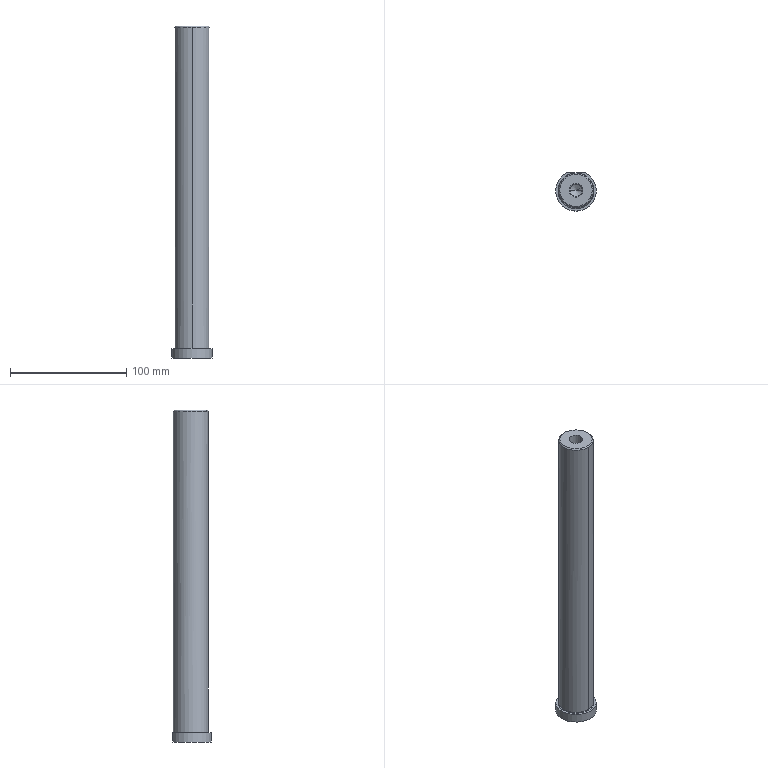Part | Creo | 1 solid | 21 faces | box 35 x 33 x 286 mm | volume 201353 mm3 | cylinder 7 | cone 6 | plane 4 | torus 4 | commonest cylinder face diameters 10.3 x2 12 x2 30 x2 35 x1
STEP:
#1=CARTESIAN_POINT('',(160.124,-246.505,-296.));
#2=VERTEX_POINT('',#1);
#3=CARTESIAN_POINT('',(152.,-279.505,-296.));
#4=VERTEX_POINT('',#3);
#5=CARTESIAN_POINT('',(152.,-262.005,-296.));
#6=DIRECTION('',(0.,0.,-1.));
#7=DIRECTION('',(0.4642,0.8857,0.));
#8=AXIS2_PLACEMENT_3D('',#5,#6,#7);
#9=CIRCLE('',#8,17.5);
#10=EDGE_CURVE('',#2,#4,#9,.T.);
#11=ORIENTED_EDGE('',*,*,#10,.F.);
#12=CARTESIAN_POINT('',(143.876,-246.505,-296.));
#13=VERTEX_POINT('',#12);
#14=CARTESIAN_POINT('',(160.124,-246.505,-296.));
#15=DIRECTION('',(-1.,0.,0.));
#16=VECTOR('',#15,16.248);
#17=LINE('',#14,#16);
#18=EDGE_CURVE('',#2,#13,#17,.T.);
#19=ORIENTED_EDGE('',*,*,#18,.T.);
#20=CARTESIAN_POINT('',(152.,-262.005,-296.));
#21=DIRECTION('',(0.,0.,-1.));
#22=DIRECTION('',(0.,-1.,0.));
#23=AXIS2_PLACEMENT_3D('',#20,#21,#22);
#24=CIRCLE('',#23,17.5);
#25=EDGE_CURVE('',#4,#13,#24,.T.);
#26=ORIENTED_EDGE('',*,*,#25,.F.);
#27=EDGE_LOOP('',(#11,#19,#26));
#28=FACE_OUTER_BOUND('',#27,.F.);
#29=CARTESIAN_POINT('',(152.,-262.005,-296.));
#30=DIRECTION('',(0.,0.,1.));
#31=DIRECTION('',(0.,1.,0.));
#32=AXIS2_PLACEMENT_3D('',#29,#30,#31);
#33=PLANE('',#32);
#34=ADVANCED_FACE('',(#28),#33,.F.);
#35=CARTESIAN_POINT('',(160.124,-246.505,-288.));
#36=VERTEX_POINT('',#35);
#37=CARTESIAN_POINT('',(160.124,-246.505,-296.));
#38=DIRECTION('',(0.,0.,1.));
#39=VECTOR('',#38,8.);
#40=LINE('',#37,#39);
#41=EDGE_CURVE('',#2,#36,#40,.T.);
#42=ORIENTED_EDGE('',*,*,#41,.F.);
#43=ORIENTED_EDGE('',*,*,#10,.T.);
#44=ORIENTED_EDGE('',*,*,#25,.T.);
#45=CARTESIAN_POINT('',(143.876,-246.505,-288.));
#46=VERTEX_POINT('',#45);
#47=CARTESIAN_POINT('',(143.876,-246.505,-288.));
#48=DIRECTION('',(0.,0.,-1.));
#49=VECTOR('',#48,8.);
#50=LINE('',#47,#49);
#51=EDGE_CURVE('',#46,#13,#50,.T.);
#52=ORIENTED_EDGE('',*,*,#51,.F.);
#53=CARTESIAN_POINT('',(152.,-279.505,-288.));
#54=VERTEX_POINT('',#53);
#55=CARTESIAN_POINT('',(152.,-262.005,-288.));
#56=DIRECTION('',(0.,0.,1.));
#57=DIRECTION('',(-0.4642,0.8857,0.));
#58=AXIS2_PLACEMENT_3D('',#55,#56,#57);
#59=CIRCLE('',#58,17.5);
#60=EDGE_CURVE('',#46,#54,#59,.T.);
#61=ORIENTED_EDGE('',*,*,#60,.T.);
#62=CARTESIAN_POINT('',(152.,-262.005,-288.));
#63=DIRECTION('',(0.,0.,1.));
#64=DIRECTION('',(0.,-1.,0.));
#65=AXIS2_PLACEMENT_3D('',#62,#63,#64);
#66=CIRCLE('',#65,17.5);
#67=EDGE_CURVE('',#54,#36,#66,.T.);
#68=ORIENTED_EDGE('',*,*,#67,.T.);
#69=EDGE_LOOP('',(#42,#43,#44,#52,#61,#68));
#70=FACE_OUTER_BOUND('',#69,.F.);
#71=CARTESIAN_POINT('',(152.,-262.005,-312.25));
#72=DIRECTION('',(0.,0.,1.));
#73=DIRECTION('',(0.,1.,0.));
#74=AXIS2_PLACEMENT_3D('',#71,#72,#73);
#75=CYLINDRICAL_SURFACE('',#74,17.5);
#76=ADVANCED_FACE('',(#70),#75,.T.);
#77=ORIENTED_EDGE('',*,*,#41,.T.);
#78=CARTESIAN_POINT('',(152.,-246.505,-288.));
#79=VERTEX_POINT('',#78);
#80=CARTESIAN_POINT('',(152.,-246.505,-288.));
#81=DIRECTION('',(1.,0.,0.));
#82=VECTOR('',#81,8.124);
#83=LINE('',#80,#82);
#84=EDGE_CURVE('',#79,#36,#83,.T.);
#85=ORIENTED_EDGE('',*,*,#84,.F.);
#86=CARTESIAN_POINT('',(143.876,-246.505,-288.));
#87=DIRECTION('',(1.,0.,0.));
#88=VECTOR('',#87,8.124);
#89=LINE('',#86,#88);
#90=EDGE_CURVE('',#46,#79,#89,.T.);
#91=ORIENTED_EDGE('',*,*,#90,.F.);
#92=ORIENTED_EDGE('',*,*,#51,.T.);
#93=ORIENTED_EDGE('',*,*,#18,.F.);
#94=EDGE_LOOP('',(#77,#85,#91,#92,#93));
#95=FACE_OUTER_BOUND('',#94,.F.);
#96=CARTESIAN_POINT('',(152.,-246.505,-297.));
#97=DIRECTION('',(0.,-1.,0.));
#98=DIRECTION('',(0.,0.,1.));
#99=AXIS2_PLACEMENT_3D('',#96,#97,#98);
#100=PLANE('',#99);
#101=ADVANCED_FACE('',(#95),#100,.F.);
#102=ORIENTED_EDGE('',*,*,#60,.F.);
#103=ORIENTED_EDGE('',*,*,#90,.T.);
#104=CARTESIAN_POINT('',(152.,-277.505,-288.));
#105=VERTEX_POINT('',#104);
#106=CARTESIAN_POINT('',(152.,-262.005,-288.));
#107=DIRECTION('',(0.,0.,-1.));
#108=DIRECTION('',(0.,-1.,0.));
#109=AXIS2_PLACEMENT_3D('',#106,#107,#108);
#110=CIRCLE('',#109,15.5);
#111=EDGE_CURVE('',#105,#79,#110,.T.);
#112=ORIENTED_EDGE('',*,*,#111,.F.);
#113=CARTESIAN_POINT('',(152.,-262.005,-288.));
#114=DIRECTION('',(0.,0.,-1.));
#115=DIRECTION('',(0.,1.,0.));
#116=AXIS2_PLACEMENT_3D('',#113,#114,#115);
#117=CIRCLE('',#116,15.5);
#118=EDGE_CURVE('',#79,#105,#117,.T.);
#119=ORIENTED_EDGE('',*,*,#118,.F.);
#120=ORIENTED_EDGE('',*,*,#84,.T.);
#121=ORIENTED_EDGE('',*,*,#67,.F.);
#122=EDGE_LOOP('',(#102,#103,#112,#119,#120,#121));
#123=FACE_OUTER_BOUND('',#122,.F.);
#124=CARTESIAN_POINT('',(152.,-262.005,-288.));
#125=DIRECTION('',(0.,0.,1.));
#126=DIRECTION('',(0.,1.,0.));
#127=AXIS2_PLACEMENT_3D('',#124,#125,#126);
#128=PLANE('',#127);
#129=ADVANCED_FACE('',(#123),#128,.T.);
#130=ORIENTED_EDGE('',*,*,#111,.T.);
#131=CARTESIAN_POINT('',(152.,-246.858,-287.854));
#132=VERTEX_POINT('',#131);
#133=CARTESIAN_POINT('',(152.,-246.505,-287.5));
#134=DIRECTION('',(1.,0.,0.));
#135=DIRECTION('',(0.,-0.7071,-0.7071));
#136=AXIS2_PLACEMENT_3D('',#133,#134,#135);
#137=CIRCLE('',#136,0.5);
#138=EDGE_CURVE('',#132,#79,#137,.T.);
#139=ORIENTED_EDGE('',*,*,#138,.F.);
#140=CARTESIAN_POINT('',(152.,-277.151,-287.854));
#141=VERTEX_POINT('',#140);
#142=CARTESIAN_POINT('',(152.,-262.005,-287.854));
#143=DIRECTION('',(0.,0.,1.));
#144=DIRECTION('',(0.,1.,0.));
#145=AXIS2_PLACEMENT_3D('',#142,#143,#144);
#146=CIRCLE('',#145,15.146);
#147=EDGE_CURVE('',#132,#141,#146,.T.);
#148=ORIENTED_EDGE('',*,*,#147,.T.);
#149=CARTESIAN_POINT('',(152.,-277.505,-287.5));
#150=DIRECTION('',(-1.,0.,0.));
#151=DIRECTION('',(0.,0.7071,-0.7071));
#152=AXIS2_PLACEMENT_3D('',#149,#150,#151);
#153=CIRCLE('',#152,0.5);
#154=EDGE_CURVE('',#141,#105,#153,.T.);
#155=ORIENTED_EDGE('',*,*,#154,.T.);
#156=EDGE_LOOP('',(#130,#139,#148,#155));
#157=FACE_OUTER_BOUND('',#156,.F.);
#158=CARTESIAN_POINT('',(152.,-262.005,-287.5));
#159=DIRECTION('',(0.,0.,1.));
#160=DIRECTION('',(0.,1.,0.));
#161=AXIS2_PLACEMENT_3D('',#158,#159,#160);
#162=TOROIDAL_SURFACE('',#161,15.5,0.5);
#163=ADVANCED_FACE('',(#157),#162,.F.);
#164=ORIENTED_EDGE('',*,*,#118,.T.);
#165=ORIENTED_EDGE('',*,*,#154,.F.);
#166=CARTESIAN_POINT('',(152.,-262.005,-287.854));
#167=DIRECTION('',(0.,0.,1.));
#168=DIRECTION('',(0.,-1.,0.));
#169=AXIS2_PLACEMENT_3D('',#166,#167,#168);
#170=CIRCLE('',#169,15.146);
#171=EDGE_CURVE('',#141,#132,#170,.T.);
#172=ORIENTED_EDGE('',*,*,#171,.T.);
#173=ORIENTED_EDGE('',*,*,#138,.T.);
#174=EDGE_LOOP('',(#164,#165,#172,#173));
#175=FACE_OUTER_BOUND('',#174,.F.);
#176=CARTESIAN_POINT('',(152.,-262.005,-287.5));
#177=DIRECTION('',(0.,0.,1.));
#178=DIRECTION('',(0.,1.,0.));
#179=AXIS2_PLACEMENT_3D('',#176,#177,#178);
#180=TOROIDAL_SURFACE('',#179,15.5,0.5);
#181=ADVANCED_FACE('',(#175),#180,.F.);
#182=CARTESIAN_POINT('',(152.,-247.005,-287.5));
#183=VERTEX_POINT('',#182);
#184=CARTESIAN_POINT('',(152.,-277.005,-287.5));
#185=VERTEX_POINT('',#184);
#186=CARTESIAN_POINT('',(152.,-262.005,-287.5));
#187=DIRECTION('',(0.,0.,-1.));
#188=DIRECTION('',(0.,1.,0.));
#189=AXIS2_PLACEMENT_3D('',#186,#187,#188);
#190=CIRCLE('',#189,15.);
#191=EDGE_CURVE('',#183,#185,#190,.T.);
#192=ORIENTED_EDGE('',*,*,#191,.F.);
#193=CARTESIAN_POINT('',(152.,-246.505,-287.5));
#194=DIRECTION('',(1.,0.,0.));
#195=DIRECTION('',(0.,-1.,0.));
#196=AXIS2_PLACEMENT_3D('',#193,#194,#195);
#197=CIRCLE('',#196,0.5);
#198=EDGE_CURVE('',#183,#132,#197,.T.);
#199=ORIENTED_EDGE('',*,*,#198,.T.);
#200=ORIENTED_EDGE('',*,*,#171,.F.);
#201=CARTESIAN_POINT('',(152.,-277.505,-287.5));
#202=DIRECTION('',(-1.,0.,0.));
#203=DIRECTION('',(0.,1.,0.));
#204=AXIS2_PLACEMENT_3D('',#201,#202,#203);
#205=CIRCLE('',#204,0.5);
#206=EDGE_CURVE('',#185,#141,#205,.T.);
#207=ORIENTED_EDGE('',*,*,#206,.F.);
#208=EDGE_LOOP('',(#192,#199,#200,#207));
#209=FACE_OUTER_BOUND('',#208,.F.);
#210=CARTESIAN_POINT('',(152.,-262.005,-287.5));
#211=DIRECTION('',(0.,0.,1.));
#212=DIRECTION('',(0.,1.,0.));
#213=AXIS2_PLACEMENT_3D('',#210,#211,#212);
#214=TOROIDAL_SURFACE('',#213,15.5,0.5);
#215=ADVANCED_FACE('',(#209),#214,.F.);
#216=ORIENTED_EDGE('',*,*,#191,.T.);
#217=CARTESIAN_POINT('',(152.,-277.005,-11.));
#218=VERTEX_POINT('',#217);
#219=CARTESIAN_POINT('',(152.,-277.005,-287.5));
#220=DIRECTION('',(0.,0.,1.));
#221=VECTOR('',#220,276.5);
#222=LINE('',#219,#221);
#223=EDGE_CURVE('',#185,#218,#222,.T.);
#224=ORIENTED_EDGE('',*,*,#223,.T.);
#225=CARTESIAN_POINT('',(167.,-262.005,-11.));
#226=VERTEX_POINT('',#225);
#227=CARTESIAN_POINT('',(152.,-262.005,-11.));
#228=DIRECTION('',(0.,0.,1.));
#229=DIRECTION('',(0.,-1.,0.));
#230=AXIS2_PLACEMENT_3D('',#227,#228,#229);
#231=CIRCLE('',#230,15.);
#232=EDGE_CURVE('',#218,#226,#231,.T.);
#233=ORIENTED_EDGE('',*,*,#232,.T.);
#234=CARTESIAN_POINT('',(152.,-247.005,-11.));
#235=VERTEX_POINT('',#234);
#236=CARTESIAN_POINT('',(152.,-262.005,-11.));
#237=DIRECTION('',(0.,0.,1.));
#238=DIRECTION('',(1.,0.,0.));
#239=AXIS2_PLACEMENT_3D('',#236,#237,#238);
#240=CIRCLE('',#239,15.);
#241=EDGE_CURVE('',#226,#235,#240,.T.);
#242=ORIENTED_EDGE('',*,*,#241,.T.);
#243=CARTESIAN_POINT('',(152.,-247.005,-287.5));
#244=DIRECTION('',(0.,0.,1.));
#245=VECTOR('',#244,276.5);
#246=LINE('',#243,#245);
#247=EDGE_CURVE('',#183,#235,#246,.T.);
#248=ORIENTED_EDGE('',*,*,#247,.F.);
#249=EDGE_LOOP('',(#216,#224,#233,#242,#248));
#250=FACE_OUTER_BOUND('',#249,.F.);
#251=CARTESIAN_POINT('',(152.,-262.005,-352.25));
#252=DIRECTION('',(0.,0.,1.));
#253=DIRECTION('',(0.,1.,0.));
#254=AXIS2_PLACEMENT_3D('',#251,#252,#253);
#255=CYLINDRICAL_SURFACE('',#254,15.);
#256=ADVANCED_FACE('',(#250),#255,.T.);
#257=CARTESIAN_POINT('',(152.,-262.005,-287.5));
#258=DIRECTION('',(0.,0.,-1.));
#259=DIRECTION('',(0.,-1.,0.));
#260=AXIS2_PLACEMENT_3D('',#257,#258,#259);
#261=CIRCLE('',#260,15.);
#262=EDGE_CURVE('',#185,#183,#261,.T.);
#263=ORIENTED_EDGE('',*,*,#262,.T.);
#264=ORIENTED_EDGE('',*,*,#247,.T.);
#265=CARTESIAN_POINT('',(137.,-262.005,-11.));
#266=VERTEX_POINT('',#265);
#267=CARTESIAN_POINT('',(152.,-262.005,-11.));
#268=DIRECTION('',(0.,0.,1.));
#269=DIRECTION('',(0.,1.,0.));
#270=AXIS2_PLACEMENT_3D('',#267,#268,#269);
#271=CIRCLE('',#270,15.);
#272=EDGE_CURVE('',#235,#266,#271,.T.);
#273=ORIENTED_EDGE('',*,*,#272,.T.);
#274=CARTESIAN_POINT('',(152.,-262.005,-11.));
#275=DIRECTION('',(0.,0.,1.));
#276=DIRECTION('',(-1.,0.,0.));
#277=AXIS2_PLACEMENT_3D('',#274,#275,#276);
#278=CIRCLE('',#277,15.);
#279=EDGE_CURVE('',#266,#218,#278,.T.);
#280=ORIENTED_EDGE('',*,*,#279,.T.);
#281=ORIENTED_EDGE('',*,*,#223,.F.);
#282=EDGE_LOOP('',(#263,#264,#273,#280,#281));
#283=FACE_OUTER_BOUND('',#282,.F.);
#284=CARTESIAN_POINT('',(152.,-262.005,-352.25));
#285=DIRECTION('',(0.,0.,1.));
#286=DIRECTION('',(0.,1.,0.));
#287=AXIS2_PLACEMENT_3D('',#284,#285,#286);
#288=CYLINDRICAL_SURFACE('',#287,15.);
#289=ADVANCED_FACE('',(#283),#288,.T.);
#290=ORIENTED_EDGE('',*,*,#262,.F.);
#291=ORIENTED_EDGE('',*,*,#206,.T.);
#292=ORIENTED_EDGE('',*,*,#147,.F.);
#293=ORIENTED_EDGE('',*,*,#198,.F.);
#294=EDGE_LOOP('',(#290,#291,#292,#293));
#295=FACE_OUTER_BOUND('',#294,.F.);
#296=CARTESIAN_POINT('',(152.,-262.005,-287.5));
#297=DIRECTION('',(0.,0.,1.));
#298=DIRECTION('',(0.,1.,0.));
#299=AXIS2_PLACEMENT_3D('',#296,#297,#298);
#300=TOROIDAL_SURFACE('',#299,15.5,0.5);
#301=ADVANCED_FACE('',(#295),#300,.F.);
#302=ORIENTED_EDGE('',*,*,#241,.F.);
#303=CARTESIAN_POINT('',(166.,-262.005,-10.));
#304=VERTEX_POINT('',#303);
#305=CARTESIAN_POINT('',(166.,-262.005,-10.));
#306=DIRECTION('',(0.7071,0.,-0.7071));
#307=VECTOR('',#306,1.414);
#308=LINE('',#305,#307);
#309=EDGE_CURVE('',#304,#226,#308,.T.);
#310=ORIENTED_EDGE('',*,*,#309,.F.);
#311=CARTESIAN_POINT('',(138.,-262.005,-10.));
#312=VERTEX_POINT('',#311);
#313=CARTESIAN_POINT('',(152.,-262.005,-10.));
#314=DIRECTION('',(0.,0.,1.));
#315=DIRECTION('',(1.,0.,0.));
#316=AXIS2_PLACEMENT_3D('',#313,#314,#315);
#317=CIRCLE('',#316,14.);
#318=EDGE_CURVE('',#304,#312,#317,.T.);
#319=ORIENTED_EDGE('',*,*,#318,.T.);
#320=CARTESIAN_POINT('',(138.,-262.005,-10.));
#321=DIRECTION('',(-0.7071,0.,-0.7071));
#322=VECTOR('',#321,1.414);
#323=LINE('',#320,#322);
#324=EDGE_CURVE('',#312,#266,#323,.T.);
#325=ORIENTED_EDGE('',*,*,#324,.T.);
#326=ORIENTED_EDGE('',*,*,#272,.F.);
#327=EDGE_LOOP('',(#302,#310,#319,#325,#326));
#328=FACE_OUTER_BOUND('',#327,.F.);
#329=CARTESIAN_POINT('',(152.,-262.005,-10.5));
#330=DIRECTION('',(0.,0.,-1.));
#331=DIRECTION('',(1.,0.,0.));
#332=AXIS2_PLACEMENT_3D('',#329,#330,#331);
#333=CONICAL_SURFACE('',#332,14.5,45.);
#334=ADVANCED_FACE('',(#328),#333,.T.);
#335=ORIENTED_EDGE('',*,*,#279,.F.);
#336=ORIENTED_EDGE('',*,*,#324,.F.);
#337=CARTESIAN_POINT('',(152.,-262.005,-10.));
#338=DIRECTION('',(0.,0.,1.));
#339=DIRECTION('',(-1.,0.,0.));
#340=AXIS2_PLACEMENT_3D('',#337,#338,#339);
#341=CIRCLE('',#340,14.);
#342=EDGE_CURVE('',#312,#304,#341,.T.);
#343=ORIENTED_EDGE('',*,*,#342,.T.);
#344=ORIENTED_EDGE('',*,*,#309,.T.);
#345=ORIENTED_EDGE('',*,*,#232,.F.);
#346=EDGE_LOOP('',(#335,#336,#343,#344,#345));
#347=FACE_OUTER_BOUND('',#346,.F.);
#348=CARTESIAN_POINT('',(152.,-262.005,-10.5));
#349=DIRECTION('',(0.,0.,-1.));
#350=DIRECTION('',(1.,0.,0.));
#351=AXIS2_PLACEMENT_3D('',#348,#349,#350);
#352=CONICAL_SURFACE('',#351,14.5,45.);
#353=ADVANCED_FACE('',(#347),#352,.T.);
#354=ORIENTED_EDGE('',*,*,#318,.F.);
#355=ORIENTED_EDGE('',*,*,#342,.F.);
#356=EDGE_LOOP('',(#354,#355));
#357=FACE_OUTER_BOUND('',#356,.F.);
#358=CARTESIAN_POINT('',(158.,-262.005,-10.));
#359=VERTEX_POINT('',#358);
#360=CARTESIAN_POINT('',(146.,-262.005,-10.));
#361=VERTEX_POINT('',#360);
#362=CARTESIAN_POINT('',(152.,-262.005,-10.));
#363=DIRECTION('',(0.,0.,-1.));
#364=DIRECTION('',(1.,0.,0.));
#365=AXIS2_PLACEMENT_3D('',#362,#363,#364);
#366=CIRCLE('',#365,6.);
#367=EDGE_CURVE('',#359,#361,#366,.T.);
#368=ORIENTED_EDGE('',*,*,#367,.F.);
#369=CARTESIAN_POINT('',(152.,-262.005,-10.));
#370=DIRECTION('',(0.,0.,-1.));
#371=DIRECTION('',(-1.,0.,0.));
#372=AXIS2_PLACEMENT_3D('',#369,#370,#371);
#373=CIRCLE('',#372,6.);
#374=EDGE_CURVE('',#361,#359,#373,.T.);
#375=ORIENTED_EDGE('',*,*,#374,.F.);
#376=EDGE_LOOP('',(#368,#375));
#377=FACE_BOUND('',#376,.F.);
#378=CARTESIAN_POINT('',(152.,-262.005,-10.));
#379=DIRECTION('',(0.,0.,1.));
#380=DIRECTION('',(0.,1.,0.));
#381=AXIS2_PLACEMENT_3D('',#378,#379,#380);
#382=PLANE('',#381);
#383=ADVANCED_FACE('',(#357,#377),#382,.T.);
#384=CARTESIAN_POINT('',(146.,-262.005,-28.));
#385=VERTEX_POINT('',#384);
#386=CARTESIAN_POINT('',(158.,-262.005,-28.));
#387=VERTEX_POINT('',#386);
#388=CARTESIAN_POINT('',(152.,-262.005,-28.));
#389=DIRECTION('',(0.,0.,1.));
#390=DIRECTION('',(-1.,0.,0.));
#391=AXIS2_PLACEMENT_3D('',#388,#389,#390);
#392=CIRCLE('',#391,6.);
#393=EDGE_CURVE('',#385,#387,#392,.T.);
#394=ORIENTED_EDGE('',*,*,#393,.T.);
#395=CARTESIAN_POINT('',(158.,-262.005,-28.));
#396=DIRECTION('',(0.,0.,1.));
#397=VECTOR('',#396,18.);
#398=LINE('',#395,#397);
#399=EDGE_CURVE('',#387,#359,#398,.T.);
#400=ORIENTED_EDGE('',*,*,#399,.T.);
#401=ORIENTED_EDGE('',*,*,#367,.T.);
#402=CARTESIAN_POINT('',(146.,-262.005,-28.));
#403=DIRECTION('',(0.,0.,1.));
#404=VECTOR('',#403,18.);
#405=LINE('',#402,#404);
#406=EDGE_CURVE('',#385,#361,#405,.T.);
#407=ORIENTED_EDGE('',*,*,#406,.F.);
#408=EDGE_LOOP('',(#394,#400,#401,#407));
#409=FACE_OUTER_BOUND('',#408,.F.);
#410=CARTESIAN_POINT('',(152.,-262.005,-28.));
#411=DIRECTION('',(0.,0.,1.));
#412=DIRECTION('',(-1.,0.,0.));
#413=AXIS2_PLACEMENT_3D('',#410,#411,#412);
#414=CYLINDRICAL_SURFACE('',#413,6.);
#415=ADVANCED_FACE('',(#409),#414,.F.);
#416=CARTESIAN_POINT('',(157.15,-262.005,-28.85));
#417=VERTEX_POINT('',#416);
#418=CARTESIAN_POINT('',(146.85,-262.005,-28.85));
#419=VERTEX_POINT('',#418);
#420=CARTESIAN_POINT('',(152.,-262.005,-28.85));
#421=DIRECTION('',(0.,0.,-1.));
#422=DIRECTION('',(1.,0.,0.));
#423=AXIS2_PLACEMENT_3D('',#420,#421,#422);
#424=CIRCLE('',#423,5.15);
#425=EDGE_CURVE('',#417,#419,#424,.T.);
#426=ORIENTED_EDGE('',*,*,#425,.F.);
#427=CARTESIAN_POINT('',(157.15,-262.005,-28.85));
#428=DIRECTION('',(0.7071,0.,0.7071));
#429=VECTOR('',#428,1.202);
#430=LINE('',#427,#429);
#431=EDGE_CURVE('',#417,#387,#430,.T.);
#432=ORIENTED_EDGE('',*,*,#431,.T.);
#433=ORIENTED_EDGE('',*,*,#393,.F.);
#434=CARTESIAN_POINT('',(146.85,-262.005,-28.85));
#435=DIRECTION('',(-0.7071,0.,0.7071));
#436=VECTOR('',#435,1.202);
#437=LINE('',#434,#436);
#438=EDGE_CURVE('',#419,#385,#437,.T.);
#439=ORIENTED_EDGE('',*,*,#438,.F.);
#440=EDGE_LOOP('',(#426,#432,#433,#439));
#441=FACE_OUTER_BOUND('',#440,.F.);
#442=CARTESIAN_POINT('',(152.,-262.005,-28.425));
#443=DIRECTION('',(0.,0.,1.));
#444=DIRECTION('',(-1.,0.,0.));
#445=AXIS2_PLACEMENT_3D('',#442,#443,#444);
#446=CONICAL_SURFACE('',#445,5.575,45.);
#447=ADVANCED_FACE('',(#441),#446,.F.);
#448=CARTESIAN_POINT('',(146.85,-262.005,-34.));
#449=VERTEX_POINT('',#448);
#450=CARTESIAN_POINT('',(157.15,-262.005,-34.));
#451=VERTEX_POINT('',#450);
#452=CARTESIAN_POINT('',(152.,-262.005,-34.));
#453=DIRECTION('',(0.,0.,1.));
#454=DIRECTION('',(-1.,0.,0.));
#455=AXIS2_PLACEMENT_3D('',#452,#453,#454);
#456=CIRCLE('',#455,5.15);
#457=EDGE_CURVE('',#449,#451,#456,.T.);
#458=ORIENTED_EDGE('',*,*,#457,.T.);
#459=CARTESIAN_POINT('',(157.15,-262.005,-28.85));
#460=DIRECTION('',(0.,0.,-1.));
#461=VECTOR('',#460,5.15);
#462=LINE('',#459,#461);
#463=EDGE_CURVE('',#417,#451,#462,.T.);
#464=ORIENTED_EDGE('',*,*,#463,.F.);
#465=ORIENTED_EDGE('',*,*,#425,.T.);
#466=CARTESIAN_POINT('',(146.85,-262.005,-28.85));
#467=DIRECTION('',(0.,0.,-1.));
#468=VECTOR('',#467,5.15);
#469=LINE('',#466,#468);
#470=EDGE_CURVE('',#419,#449,#469,.T.);
#471=ORIENTED_EDGE('',*,*,#470,.T.);
#472=EDGE_LOOP('',(#458,#464,#465,#471));
#473=FACE_OUTER_BOUND('',#472,.F.);
#474=CARTESIAN_POINT('',(152.,-262.005,-10.));
#475=DIRECTION('',(0.,0.,-1.));
#476=DIRECTION('',(1.,0.,0.));
#477=AXIS2_PLACEMENT_3D('',#474,#475,#476);
#478=CYLINDRICAL_SURFACE('',#477,5.15);
#479=ADVANCED_FACE('',(#473),#478,.F.);
#480=ORIENTED_EDGE('',*,*,#457,.F.);
#481=CARTESIAN_POINT('',(152.,-262.005,-37.094));
#482=VERTEX_POINT('',#481);
#483=CARTESIAN_POINT('',(152.,-262.005,-37.094));
#484=DIRECTION('',(-0.8572,0.,0.515));
#485=VECTOR('',#484,6.008);
#486=LINE('',#483,#485);
#487=EDGE_CURVE('',#482,#449,#486,.T.);
#488=ORIENTED_EDGE('',*,*,#487,.F.);
#489=CARTESIAN_POINT('',(152.,-262.005,-37.094));
#490=DIRECTION('',(0.8572,0.,0.515));
#491=VECTOR('',#490,6.008);
#492=LINE('',#489,#491);
#493=EDGE_CURVE('',#482,#451,#492,.T.);
#494=ORIENTED_EDGE('',*,*,#493,.T.);
#495=EDGE_LOOP('',(#480,#488,#494));
#496=FACE_OUTER_BOUND('',#495,.F.);
#497=CARTESIAN_POINT('',(152.,-262.005,-35.458));
#498=DIRECTION('',(0.,0.,1.));
#499=DIRECTION('',(-1.,0.,0.));
#500=AXIS2_PLACEMENT_3D('',#497,#498,#499);
#501=CONICAL_SURFACE('',#500,2.724,59.);
#502=ADVANCED_FACE('',(#496),#501,.F.);
#503=CARTESIAN_POINT('',(152.,-262.005,-34.));
#504=DIRECTION('',(0.,0.,1.));
#505=DIRECTION('',(1.,0.,0.));
#506=AXIS2_PLACEMENT_3D('',#503,#504,#505);
#507=CIRCLE('',#506,5.15);
#508=EDGE_CURVE('',#451,#449,#507,.T.);
#509=ORIENTED_EDGE('',*,*,#508,.F.);
#510=ORIENTED_EDGE('',*,*,#493,.F.);
#511=ORIENTED_EDGE('',*,*,#487,.T.);
#512=EDGE_LOOP('',(#509,#510,#511));
#513=FACE_OUTER_BOUND('',#512,.F.);
#514=CARTESIAN_POINT('',(152.,-262.005,-35.458));
#515=DIRECTION('',(0.,0.,1.));
#516=DIRECTION('',(-1.,0.,0.));
#517=AXIS2_PLACEMENT_3D('',#514,#515,#516);
#518=CONICAL_SURFACE('',#517,2.724,59.);
#519=ADVANCED_FACE('',(#513),#518,.F.);
#520=ORIENTED_EDGE('',*,*,#508,.T.);
#521=ORIENTED_EDGE('',*,*,#470,.F.);
#522=CARTESIAN_POINT('',(152.,-262.005,-28.85));
#523=DIRECTION('',(0.,0.,-1.));
#524=DIRECTION('',(-1.,0.,0.));
#525=AXIS2_PLACEMENT_3D('',#522,#523,#524);
#526=CIRCLE('',#525,5.15);
#527=EDGE_CURVE('',#419,#417,#526,.T.);
#528=ORIENTED_EDGE('',*,*,#527,.T.);
#529=ORIENTED_EDGE('',*,*,#463,.T.);
#530=EDGE_LOOP('',(#520,#521,#528,#529));
#531=FACE_OUTER_BOUND('',#530,.F.);
#532=CARTESIAN_POINT('',(152.,-262.005,-10.));
#533=DIRECTION('',(0.,0.,-1.));
#534=DIRECTION('',(1.,0.,0.));
#535=AXIS2_PLACEMENT_3D('',#532,#533,#534);
#536=CYLINDRICAL_SURFACE('',#535,5.15);
#537=ADVANCED_FACE('',(#531),#536,.F.);
#538=ORIENTED_EDGE('',*,*,#527,.F.);
#539=ORIENTED_EDGE('',*,*,#438,.T.);
#540=CARTESIAN_POINT('',(152.,-262.005,-28.));
#541=DIRECTION('',(0.,0.,1.));
#542=DIRECTION('',(1.,0.,0.));
#543=AXIS2_PLACEMENT_3D('',#540,#541,#542);
#544=CIRCLE('',#543,6.);
#545=EDGE_CURVE('',#387,#385,#544,.T.);
#546=ORIENTED_EDGE('',*,*,#545,.F.);
#547=ORIENTED_EDGE('',*,*,#431,.F.);
#548=EDGE_LOOP('',(#538,#539,#546,#547));
#549=FACE_OUTER_BOUND('',#548,.F.);
#550=CARTESIAN_POINT('',(152.,-262.005,-28.425));
#551=DIRECTION('',(0.,0.,1.));
#552=DIRECTION('',(-1.,0.,0.));
#553=AXIS2_PLACEMENT_3D('',#550,#551,#552);
#554=CONICAL_SURFACE('',#553,5.575,45.);
#555=ADVANCED_FACE('',(#549),#554,.F.);
#556=ORIENTED_EDGE('',*,*,#545,.T.);
#557=ORIENTED_EDGE('',*,*,#406,.T.);
#558=ORIENTED_EDGE('',*,*,#374,.T.);
#559=ORIENTED_EDGE('',*,*,#399,.F.);
#560=EDGE_LOOP('',(#556,#557,#558,#559));
#561=FACE_OUTER_BOUND('',#560,.F.);
#562=CARTESIAN_POINT('',(152.,-262.005,-28.));
#563=DIRECTION('',(0.,0.,1.));
#564=DIRECTION('',(-1.,0.,0.));
#565=AXIS2_PLACEMENT_3D('',#562,#563,#564);
#566=CYLINDRICAL_SURFACE('',#565,6.);
#567=ADVANCED_FACE('',(#561),#566,.F.);
#568=CLOSED_SHELL('',(#34,#76,#101,#129,#163,#181,#215,#256,#289,#301,#334,#353,#383,#415,#447,#479,#502,#519,#537,#555,#567));
#569=MANIFOLD_SOLID_BREP('',#568);
#570=(LENGTH_UNIT()NAMED_UNIT(*)SI_UNIT(.MILLI.,.METRE.));
#571=UNCERTAINTY_MEASURE_WITH_UNIT(LENGTH_MEASURE(0.029),#570,'','');
#572=(NAMED_UNIT(*)PLANE_ANGLE_UNIT()SI_UNIT($,.RADIAN.));
#573=PLANE_ANGLE_MEASURE_WITH_UNIT(PLANE_ANGLE_MEASURE(0.01745),#572);
#574=(CONVERSION_BASED_UNIT('DEGREE',#573)NAMED_UNIT(*)PLANE_ANGLE_UNIT());
#575=(NAMED_UNIT(*)SI_UNIT($,.STERADIAN.)SOLID_ANGLE_UNIT());
#576=(GEOMETRIC_REPRESENTATION_CONTEXT(3)GLOBAL_UNCERTAINTY_ASSIGNED_CONTEXT((#571))GLOBAL_UNIT_ASSIGNED_CONTEXT((#570,#574,#575))REPRESENTATION_CONTEXT('',''));
#577=ADVANCED_BREP_SHAPE_REPRESENTATION('',(#569),#576);